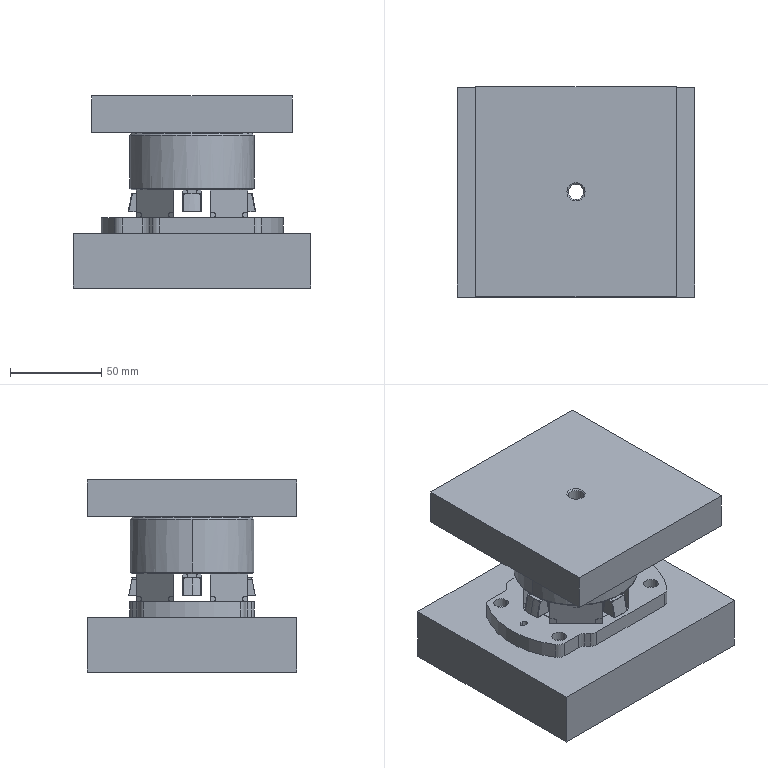NC program | NX | posted with a generic post | part box 130 x 115 x 105.2 mm
Whole program:
N10 G17 G21 G94 G90
(125 , TOOL : ER25-D2.5-23)
N12 T14 M6
N14 G54
N16 G17 G0 G90 X-40.729 Y0. B0. C0. S6500 M3
N18 G43 Z67. H14
N20 G94 G1 Z0.5 F4500.
N22 X-41.25 Z0.473 F1500.
N24 X-39.75 Z0.394
N26 X-41.25 Z0.315
N28 X-39.75 Z0.237
N30 X-41.25 Z0.158
N32 X-39.75 Z0.08
N34 X-41.25 Z0.001
N36 X-39.75 Z-0.078
N38 X-41.25 Z-0.156
N40 X-39.75 Z-0.235
N42 X-41.25 Z-0.313
N44 X-39.75 Z-0.392
N46 X-41.25 Z-0.471
N48 X-39.75 Z-0.549
N50 X-41.25 Z-0.628
N52 X-39.75 Z-0.706
N54 X-41.25 Z-0.785
N56 X-39.75 Z-0.864
N58 X-41.25 Z-0.942
N60 X-39.75 Z-1.021
N62 X-41.25 Z-1.1
N64 X-39.75 Z-1.178
N66 X-41.25 Z-1.257
N68 X-39.75 Z-1.335
N70 X-41.25 Z-1.414
N72 X-39.75 Z-1.493
N74 X-41.25 Z-1.571
N76 X-39.75 Z-1.65
N78 X-41.25 Z-1.728
N80 X-39.75 Z-1.807
N82 X-41.25 Z-1.886
N84 X-39.75 Z-1.964
N86 X-41.25 Z-2.043
N88 X-39.75 Z-2.121
N90 X-41.25 Z-2.2
N92 X-39.75 Z-2.279
N94 X-41.25 Z-2.357
N96 X-39.75 Z-2.436
N98 X-41.25 Z-2.515
N100 X-39.75 Z-2.593
N102 X-41.25 Z-2.672
N104 X-39.75 Z-2.75
N106 X-41.25 Z-2.829
N108 X-39.75 Z-2.908
N110 X-41.25 Z-2.986
N112 X-39.75 Z-3.065
N114 X-41.25 Z-3.143
N116 X-39.75 Z-3.222
N118 X-41.25 Z-3.301
N120 X-39.75 Z-3.379
N122 X-41.25 Z-3.458
N124 X-39.75 Z-3.536
N126 X-41.25 Z-3.615
N128 X-39.75 Z-3.694
N130 X-41.25 Z-3.772
N132 X-39.75 Z-3.851
N134 X-41.25 Z-3.93
N136 X-39.75 Z-4.008
N138 X-41.25 Z-4.087
N140 X-39.75 Z-4.165
N142 X-41.25 Z-4.244
N144 X-39.75 Z-4.323
N146 X-41.25 Z-4.401
N148 X-39.75 Z-4.48
N150 X-41.25 Z-4.558
N152 X-39.75 Z-4.637
N154 X-41.25 Z-4.716
N156 X-39.75 Z-4.794
N158 X-41.25 Z-4.873
N160 X-39.75 Z-4.952
N162 X-41.25 Z-5.03
N164 X-39.75 Z-5.109
N166 X-41.25 Z-5.187
N168 X-39.75 Z-5.266
N170 X-41.25 Z-5.345
N172 X-39.75 Z-5.423
N174 X-41.25 Z-5.502
N176 X-39.75 Z-5.58
N178 X-41.25 Z-5.659
N180 X-39.75 Z-5.738
N182 X-41.25 Z-5.816
N184 X-39.75 Z-5.895
N186 X-41.25 Z-5.973
N188 X-39.75 Z-6.052
N190 X-41.25 Z-6.131
N192 X-39.75 Z-6.209
N194 X-41.25 Z-6.288
N196 X-39.75 Z-6.367
N198 X-41.25 Z-6.445
N200 X-39.75 Z-6.524
N202 X-41.25 Z-6.602
N204 X-39.75 Z-6.681
N206 X-41.25 Z-6.76
N208 X-39.75 Z-6.838
N210 X-41.25 Z-6.917
N212 X-39.75 Z-6.995
N214 X-41.25 Z-7.074
N216 X-39.75 Z-7.153
N218 X-41.25 Z-7.231
N220 X-39.75 Z-7.31
N222 X-41.25 Z-7.388
N224 X-39.75 Z-7.467
N226 X-41.25 Z-7.546
N228 X-39.75 Z-7.624
N230 X-41.25 Z-7.703
N232 X-39.75 Z-7.782
N234 X-41.25 Z-7.86
N236 X-39.75 Z-7.939
N238 X-41.25 Z-8.017
N240 X-39.75 Z-8.096
N242 X-41.25 Z-8.175
N244 X-39.75 Z-8.253
N246 X-41.25 Z-8.332
N248 X-39.75 Z-8.41
N250 X-41.25 Z-8.489
N252 X-39.75 Z-8.568
N254 X-41.25 Z-8.646
N256 X-39.75 Z-8.725
N258 X-41.25 Z-8.803
N260 X-39.75 Z-8.882
N262 X-41.25 Z-8.961
N264 X-40.5 Z-9.
N266 X-39.75
N268 X-41.25
N270 X-40.5
N272 X-40.
N274 Z-8.5
N276 G0 Z67.
N278 M5
(126 , TOOL : ER25-D2.5-23_G)
N280 T15 M6
N282 G54
N284 G17 G0 G90 X-40.623 Y0. B0. C0. S4934 M3
N286 G43 Z67. H15
N288 G94 G1 Z-3. F4500.
N290 G41 X-40.625 Y-0.12 F100. D15
N292 X-40.62 Y-0.159
N294 X-40.602 Y-0.194
N296 X-40.574 Y-0.222
N298 X-40.539 Y-0.24
N300 X-40.5 Y-0.245
N302 X-39.75
N304 G3 X-39.505 Y0. R0.245
N306 X-39.75 Y0.245 R0.245
N308 G1 X-41.25
N310 G3 X-41.495 Y0. R0.245
N312 X-41.25 Y-0.245 R0.245
N314 G1 X-40.5
N316 X-40.
N318 X-39.961 Y-0.24
N320 X-39.926 Y-0.222
N322 X-39.898 Y-0.194
N324 X-39.88 Y-0.159
N326 X-39.875 Y-0.12
N328 G40
N330 X-39.877 Y0.
N332 X-40.623 Y-0.005
N334 G41 X-40.625 Y-0.125
N336 X-40.62 Y-0.164
N338 X-40.602 Y-0.199
N340 X-40.574 Y-0.227
N342 X-40.539 Y-0.245
N344 X-40.5 Y-0.25
N346 X-39.75
N348 G3 X-39.5 Y0. R0.25
N350 X-39.75 Y0.25 R0.25
N352 G1 X-41.25
N354 G3 X-41.5 Y0. R0.25
N356 X-41.25 Y-0.25 R0.25
N358 G1 X-40.5
N360 X-40.
N362 X-39.961 Y-0.245
N364 X-39.926 Y-0.227
N366 X-39.898 Y-0.199
N368 X-39.88 Y-0.164
N370 X-39.875 Y-0.125
N372 G40
N374 X-39.877 Y-0.005
N376 X-40.623 Y0. Z-6. F6000.
N378 G41 X-40.625 Y-0.12 F100.
N380 X-40.62 Y-0.159
N382 X-40.602 Y-0.194
N384 X-40.574 Y-0.222
N386 X-40.539 Y-0.24
N388 X-40.5 Y-0.245
N390 X-39.75
N392 G3 X-39.505 Y0. R0.245
N394 X-39.75 Y0.245 R0.245
N396 G1 X-41.25
N398 G3 X-41.495 Y0. R0.245
N400 X-41.25 Y-0.245 R0.245
N402 G1 X-40.5
N404 X-40.
N406 X-39.961 Y-0.24
N408 X-39.926 Y-0.222
N410 X-39.898 Y-0.194
N412 X-39.88 Y-0.159
N414 X-39.875 Y-0.12
N416 G40
N418 X-39.877 Y0.
N420 X-40.623 Y-0.005
N422 G41 X-40.625 Y-0.125
N424 X-40.62 Y-0.164
N426 X-40.602 Y-0.199
N428 X-40.574 Y-0.227
N430 X-40.539 Y-0.245
N432 X-40.5 Y-0.25
N434 X-39.75
N436 G3 X-39.5 Y0. R0.25
N438 X-39.75 Y0.25 R0.25
N440 G1 X-41.25
N442 G3 X-41.5 Y0. R0.25
N444 X-41.25 Y-0.25 R0.25
N446 G1 X-40.5
N448 X-40.
N450 X-39.961 Y-0.245
N452 X-39.926 Y-0.227
N454 X-39.898 Y-0.199
N456 X-39.88 Y-0.164
N458 X-39.875 Y-0.125
N460 G40
N462 X-39.877 Y-0.005
N464 X-40.623 Y0. Z-9. F6000.
N466 G41 X-40.625 Y-0.12 F100.
N468 X-40.62 Y-0.159
N470 X-40.602 Y-0.194
N472 X-40.574 Y-0.222
N474 X-40.539 Y-0.24
N476 X-40.5 Y-0.245
N478 X-39.75
N480 G3 X-39.505 Y0. R0.245
N482 X-39.75 Y0.245 R0.245
N484 G1 X-41.25
N486 G3 X-41.495 Y0. R0.245
N488 X-41.25 Y-0.245 R0.245
N490 G1 X-40.5
N492 X-40.
N494 X-39.961 Y-0.24
N496 X-39.926 Y-0.222
N498 X-39.898 Y-0.194
N500 X-39.88 Y-0.159
N502 X-39.875 Y-0.12
N504 G40
N506 X-39.877 Y0.
N508 X-40.623 Y-0.005
N510 G41 X-40.625 Y-0.125
N512 X-40.62 Y-0.164
N514 X-40.602 Y-0.199
N516 X-40.574 Y-0.227
N518 X-40.539 Y-0.245
N520 X-40.5 Y-0.25
N522 X-39.75
N524 G3 X-39.5 Y0. R0.25
N526 X-39.75 Y0.25 R0.25
N528 G1 X-41.25
N530 G3 X-41.5 Y0. R0.25
N532 X-41.25 Y-0.25 R0.25
N534 G1 X-40.5
N536 X-40.
N538 X-39.961 Y-0.245
N540 X-39.926 Y-0.227
N542 X-39.898 Y-0.199
N544 X-39.88 Y-0.164
N546 X-39.875 Y-0.125
N548 G40
N550 X-39.877 Y-0.005
N552 G0 Z67.
N554 M5
(ADAPTIVE_MILLING , TOOL : ER25-D10-50)
N556 T04 M6
N558 G54
N560 G17 G0 G90 X61.557 Y1.041 B0. C0. S6500 M3
N562 G43 Z67. H4
N564 Z-6.
N566 G94 G1 X61.407 Y1.026 Z-6.937 F2000.
N568 X61.258 Y1.01 Z-7.308
N570 X61.109 Y0.994 Z-7.58
N572 X60.96 Y0.978 Z-7.8
N574 X60.811 Y0.963 Z-7.984
N576 X60.662 Y0.947 Z-8.142
N578 X60.512 Y0.931 Z-8.28
N580 X60.363 Y0.915 Z-8.4
N582 X60.214 Y0.899 Z-8.505
N584 X60.065 Y0.884 Z-8.598
N586 X59.916 Y0.868 Z-8.679
N588 X59.767 Y0.852 Z-8.75
N590 X59.617 Y0.836 Z-8.81
N592 X59.468 Y0.821 Z-8.862
N594 X59.319 Y0.805 Z-8.905
N596 X59.17 Y0.789 Z-8.939
N598 X59.021 Y0.773 Z-8.966
N600 X58.872 Y0.758 Z-8.985
N602 X58.722 Y0.742 Z-8.996
N604 X58.573 Y0.726 Z-9.
N606 X56.835 Y0.542
N608 G3 X56.075 Y0.057 R1.012
N610 X55.469 Y-1.557 R5.121
N612 X55.189 Y-3.496 R6.542
N614 G1 X54.855 Y-7.003
N616 X54.298 Y-10.48
N618 X53.52 Y-13.916
N620 X52.526 Y-17.295
N622 X51.318 Y-20.604
N624 X49.903 Y-23.829
N626 X48.285 Y-26.957
N628 X46.47 Y-29.976
N630 X44.468 Y-32.874
N632 X42.285 Y-35.638
N634 G2 X39.627 Y-38.203 R45.056
N636 X30.654 Y-45.533 R68.05
N638 X-44.698 Y-31.875 R54.912
N640 X-45.9 Y-30.686 R23.81
N642 G1 X-46.779 Y-29.493
N644 X-48.53 Y-26.513
N646 X-50.091 Y-23.43
N648 X-51.457 Y-20.256
N650 X-52.621 Y-17.002
N652 X-53.581 Y-13.682
N654 X-54.331 Y-10.308
N656 X-54.869 Y-6.894
N658 X-55.192 Y-3.454
N660 X-55.3 Y0.
N662 X-55.192 Y3.455
N664 X-54.868 Y6.895
N666 X-54.331 Y10.309
N668 X-53.581 Y13.683
N670 X-52.621 Y17.003
N672 X-51.456 Y20.257
N674 X-50.091 Y23.431
N676 X-48.529 Y26.514
N678 X-46.778 Y29.494
N680 G2 X-44.339 Y32.598 R57.555
N682 X-36.468 Y41.03 R68.244
N684 X39.85 Y37.753 R54.906
N686 G1 X41.244 Y36.706
N688 X42.286 Y35.637
N690 X44.466 Y32.877
N692 X46.466 Y29.983
N694 X48.278 Y26.968
N696 X49.895 Y23.844
N698 X51.31 Y20.624
N700 X52.518 Y17.319
N702 X53.513 Y13.945
N704 X54.291 Y10.515
N706 X54.85 Y7.042
N708 X55.187 Y3.54
N710 X55.3 Y0.025
N712 X55.21 Y-2.849
N714 G3 X55.811 Y-3.803 R1.029
N716 G1 X57.534 Y-4.748 Z-8.9
N718 X57.745 Y-4.864 F15000.
N720 X57.951 Y-4.988
N722 G2 X58.335 Y-5.975 R1.001
N724 G1 X57.958 Y-7.984
N726 X57.57 Y-9.991
N728 G2 X56.311 Y-14.938 R57.161
N730 X54.364 Y-20.753 R77.546
N732 X50.136 Y-29.595 R62.207
N734 X48.222 Y-32.737 R76.126
N736 G1 X45.662 Y-36.707
N738 G2 X44.586 Y-37.137 R1.
N740 G1 X44.302 Y-37.068
N742 X42.392 Y-36.605 Z-9. F2000.
N744 X42.167 Y-36.55
N746 X41.939 Y-36.506
N748 G3 X41.242 Y-36.707 R1.004
N750 G1 X40.056 Y-37.614
N752 G3 X36.023 Y-40.298 R25.388
N754 G2 X28.458 Y-45.679 R86.812
N756 X-42.013 Y-33.615 R53.839
N758 G3 X-42.38 Y-33.353 R1.719
N760 G1 X-43.678 Y-32.637
N762 X-44.774 Y-31.806
N764 G3 X-46.314 Y-32.252 R1.
N766 X-46.255 Y-33.092 Z-8.956 R1.045
N768 G1 X-45.811 Y-34.095 Z-8.9
N770 X-45.012 Y-35.895 F15000.
N772 G3 X-44.774 Y-36.227 R1.06
N774 G1 X-42.966 Y-37.885
N776 X-41.136 Y-39.519
N778 X-40.204 Y-40.315
N780 X-39.263 Y-41.103
N782 X-37.604 Y-42.468
N784 X-35.937 Y-43.824
N786 G3 X-29.941 Y-48.068 R67.977
N788 X-26.259 Y-50.265 R58.863
N790 X-20.692 Y-52.821 R51.545
N792 X-11.888 Y-55.431 R52.347
N794 X-4.629 Y-56.645 R87.095
N796 X2.098 Y-56.811 R36.217
N798 X9.998 Y-55.815 R57.149
N800 X16.942 Y-54.12 R66.102
N802 X22.299 Y-52.122 R49.474
N804 X28.844 Y-48.784 R54.765
N806 G1 X32.007 Y-46.896
N808 X35.161 Y-44.995
N810 X38.854 Y-42.703
N812 G3 X39.261 Y-42.207 R1.007
N814 G1 X39.894 Y-40.526
N816 X40.297 Y-39.439 Z-8.959 F2000.
N818 G3 X40.209 Y-38.661 Z-9. R1.
N820 X38.854 Y-38.283 R1.
N822 G1 X36.961 Y-39.041
N824 G3 X33.434 Y-41.169 R28.709
N826 G2 X25.898 Y-45.947 R97.732
N828 X-39.701 Y-34.694 R52.812
N830 G3 X-40.475 Y-34.011 R2.805
N832 G2 X-42.38 Y-33.353 R14.859
N834 G3 X-43.729 Y-34.201 R1.
N836 X-43.441 Y-35. Z-8.955 R1.044
N838 G1 X-42.742 Y-35.835 Z-8.9
N840 X-41.994 Y-36.733 F15000.
N842 X-41.236 Y-37.623
N844 X-39.689 Y-39.111
N846 X-38.134 Y-40.592
N848 G3 X-33.759 Y-44.37 R73.242
N850 X-29.403 Y-47.292 R36.344
N852 X-25.96 Y-49.209 R99.842
N854 X-20.624 Y-51.634 R55.888
N856 X-10.848 Y-54.548 R53.534
N858 G1 X-9.843 Y-54.729
N860 X-8.835 Y-54.893
N862 X-6.044 Y-55.302
N864 G3 X2.746 Y-55.629 R48.097
N866 G1 X5.461 Y-55.47
N868 G3 X10.647 Y-54.702 R37.882
N870 X19.016 Y-52.314 R72.877
N872 X26.164 Y-49.099 R47.371
N874 X33.331 Y-44.924 R163.072
N876 G1 X36.211 Y-43.139
N878 X36.353 Y-43.031
N880 X36.476 Y-42.901
N882 X37.696 Y-41.321
N884 X38.403 Y-40.397 Z-8.959 F2000.
N886 G3 X38.548 Y-39.632 Z-9. R1.
N888 X37.355 Y-38.87 R1.
N890 X33.268 Y-40.392 R11.961
N892 X27.346 Y-43.927 R432.569
N894 G2 X10.647 Y-50.521 R55.409
N896 X-37.562 Y-35.435 R51.68
N898 G3 X-38.808 Y-34.337 R8.034
N900 X-39.545 Y-34.193 R1.678
N902 G1 X-40.644 Y-33.952
N904 G3 X-41.833 Y-34.702 R1.
N906 X-41.583 Y-35.625 Z-8.949 R1.043
N908 G1 X-40.981 Y-36.386 Z-8.9
N910 X-40.286 Y-37.271 F15000.
N912 X-39.58 Y-38.148
N914 X-39.5 Y-38.222
N916 X-36.886 Y-40.358
N918 X-34.261 Y-42.481
N920 G3 X-29.456 Y-45.941 R68.449
N922 X-21.321 Y-50.19 R50.428
N924 X-16.339 Y-52.028 R78.714
N926 X-6.364 Y-54.143 R51.577
N928 X-0.164 Y-54.665 R89.323
N930 X4.023 Y-54.462 R25.809
N932 G1 X6.335 Y-54.161
N934 X8.645 Y-53.848
N936 G3 X17.791 Y-51.57 R48.335
N938 X23.442 Y-49.21 R49.142
N940 G1 X27.022 Y-47.448
N942 X30.594 Y-45.67
N944 X32.794 Y-44.544
N946 X34.991 Y-43.409
N948 G3 X35.329 Y-43.124 R1.042
N950 G1 X36.493 Y-41.585
N952 X37.188 Y-40.658 Z-8.959 F2000.
N954 G3 X37.324 Y-39.887 Z-9. R1.
N956 X36.135 Y-39.139 R1.
N958 G2 X35.149 Y-39.246 R5.011
N960 G3 X32.094 Y-40.252 R10.348
N962 X26.499 Y-43.263 R113.682
N964 G2 X13.481 Y-48.714 R59.152
N966 X-35.356 Y-36.124 R50.6
N968 G3 X-37.398 Y-34.418 R13.365
N970 X-38.066 Y-34.3 R1.369
N972 G1 X-39.188 Y-34.219
N974 G3 X-40.221 Y-34.938 R1.
N976 X-40.011 Y-35.884 Z-8.949 R1.041
N978 G1 X-39.446 Y-36.655 Z-8.9
N980 X-38.827 Y-37.506 F15000.
N982 X-38.198 Y-38.351
N984 X-38.044 Y-38.489
N986 X-34.819 Y-40.837
N988 X-31.584 Y-43.171
N990 G3 X-26.11 Y-46.671 R77.601
N992 X-20.821 Y-49.235 R44.189
N994 X-16.907 Y-50.673 R67.048
N996 X-8.393 Y-52.981 R67.15
N998 X-0.743 Y-53.574 R33.294
N1000 X6.597 Y-53.048 R84.732
N1002 X13.209 Y-51.772 R48.024
N1004 X20.174 Y-49.444 R51.333
N1006 X34.005 Y-43.516 R529.24
N1008 X34.426 Y-43.167 R1.013
N1010 G1 X35.434 Y-41.701
N1012 X36.083 Y-40.746 Z-8.959 F2000.
N1014 G3 X36.182 Y-39.966 Z-9. R1.
N1016 X35.149 Y-39.246 R1.
N1018 X33.391 Y-39.349 R86.82
N1020 X29.731 Y-40.591 R14.09
N1022 X23.318 Y-43.785 R423.321
N1024 G2 X7.788 Y-48.833 R54.739
N1026 X-33.005 Y-36.822 R49.472
N1028 G3 X-35.615 Y-34.658 R29.808
N1030 X-36.414 Y-34.3 R1.797
N1032 G1 X-37.914
N1034 G3 X-38.873 Y-35.016 R1.
N1036 X-38.678 Y-35.953 Z-8.949 R1.043
N1038 G1 X-38.122 Y-36.747 Z-8.9
N1040 X-37.021 Y-38.321 F15000.
N1042 X-36.905 Y-38.455
N1044 X-36.77 Y-38.57
N1046 X-34.249 Y-40.316
N1048 X-31.719 Y-42.049
N1050 G3 X-21.548 Y-47.706 R74.879
N1052 X-8.686 Y-51.617 R50.172
N1054 X-1.065 Y-52.413 R69.958
N1056 X5.955 Y-52.076 R39.103
N1058 X16.892 Y-49.58 R55.986
N1060 X23.525 Y-46.91 R70.317
N1062 G1 X31.699 Y-43.128
N1064 X31.868 Y-43.028
N1066 X33.6 Y-41.763
N1068 X34.553 Y-41.062 Z-8.96 F2000.
N1070 G3 X34.905 Y-40.387 Z-9. R1.
N1072 X33.909 Y-39.3 R1.
N1074 X31.774 Y-39.35 R16.816
N1076 X27.681 Y-40.676 R16.703
N1078 G1 X21.146 Y-43.668
N1080 G2 X5.545 Y-48.036 R53.459
N1082 X-31.279 Y-36.884 R48.475
N1084 G3 X-34.142 Y-34.647 R35.773
N1086 X-34.94 Y-34.3 R1.842
N1088 G1 X-36.44
N1090 G3 X-37.398 Y-35.013 R1.
N1092 X-37.208 Y-35.948 Z-8.95 R1.043
N1094 G1 X-36.656 Y-36.749 Z-8.9
N1096 X-35.597 Y-38.285 F15000.
N1098 G3 X-35.296 Y-38.57 R1.056
N1100 G1 X-27.445 Y-43.378
N1102 G3 X-17.335 Y-48.238 R54.627
N1104 X-10.45 Y-50.149 R49.024
N1106 G1 X-7.743 Y-50.694
N1108 X-5.033 Y-51.227
N1110 X-4.23 Y-51.378
N1112 X-3.424 Y-51.515
N1114 G3 X-1.393 Y-51.58 R9.81
N1116 G1 X0.749 Y-51.424
N1118 X2.89 Y-51.259
N1120 G3 X8.768 Y-50.518 R77.791
N1122 X19.552 Y-47.434 R51.222
N1124 G1 X30.074 Y-43.128
N1126 X30.183 Y-43.073
N1128 X30.287 Y-43.009
N1130 X31.981 Y-41.764
N1132 X32.93 Y-41.06 Z-8.96 F2000.
N1134 G3 X33.28 Y-40.383 Z-9. R1.
N1136 X32.284 Y-39.3 R1.
N1138 X30.037 Y-39.344 R20.664
N1140 X26.038 Y-40.515 R17.729
N1142 G1 X19.466 Y-43.268
N1144 G2 X4.363 Y-47.058 R53.087
N1146 X-29.273 Y-37.107 R47.391
N1148 G3 X-32.49 Y-34.701 R57.335
N1150 X-33.385 Y-34.3 R2.147
N1152 G1 X-35.01
N1154 G3 X-36.008 Y-35.373 R1.
N1156 X-35.521 Y-36.164 Z-8.951 R1.04
N1158 G1 X-34.71 Y-36.75 Z-8.9
N1160 X-32.8 Y-38.128 F15000.
N1162 X-31.262 Y-39.363
N1164 X-29.712 Y-40.585
N1166 G3 X-24.775 Y-43.729 R36.797
N1168 X-14.859 Y-47.939 R54.835
N1170 X-10.461 Y-49.046 R44.725
N1172 X-0.859 Y-50.146 R54.155
N1174 X11.784 Y-48.792 R52.599
N1176 X15.551 Y-47.71 R41.52
N1178 X23.273 Y-45.018 R309.641
N1180 G1 X25.8 Y-44.078
N1182 X28.324 Y-43.128
N1184 X28.448 Y-43.069
N1186 X28.566 Y-42.997
N1188 X30.234 Y-41.765
N1190 X31.182 Y-41.058 Z-8.96 F2000.
N1192 G3 X31.53 Y-40.382 Z-9. R1.
N1194 X30.534 Y-39.3 R1.
N1196 X28.293 Y-39.318 R109.815
N1198 X24.263 Y-40.359 R17.754
N1200 G1 X17.722 Y-42.844
N1202 G2 X3.121 Y-46.056 R52.472
N1204 X-27.488 Y-37.091 R46.395
N1206 G3 X-30.899 Y-34.671 R77.132
N1208 X-31.743 Y-34.3 R2.12
N1210 G1 X-33.493
N1212 G3 X-34.491 Y-35.372 R1.
N1214 X-34.005 Y-36.164 Z-8.951 R1.04
N1216 G1 X-33.194 Y-36.75 Z-8.9
N1218 X-31.283 Y-38.128 F15000.
N1220 X-28.63 Y-39.918
N1222 X-25.968 Y-41.694
N1224 G3 X-20.44 Y-44.64 R39.556
N1226 X-11.762 Y-47.631 R53.177
N1228 X-6.267 Y-48.693 R56.402
N1230 X0.575 Y-49.047 R39.156
N1232 G1 X2.003 Y-48.991
N1234 X3.431 Y-48.925
N1236 G3 X14.456 Y-46.918 R47.061
N1238 G1 X18.136 Y-45.783
N1240 X21.808 Y-44.621
N1242 X26.324 Y-43.128
N1244 X26.469 Y-43.064
N1246 X26.605 Y-42.981
N1248 X28.241 Y-41.765
N1250 X29.185 Y-41.056 Z-8.96 F2000.
N1252 G3 X29.531 Y-40.376 Z-9. R1.
N1254 X28.534 Y-39.3 R1.
N1256 X26.154 Y-39.318 R115.941
N1258 X21.947 Y-40.33 R19.912
N1260 G2 X14.623 Y-42.791 R276.472
N1262 X-2.52 Y-44.986 R48.992
N1264 X-25.984 Y-36.827 R45.591
N1266 G3 X-29.368 Y-34.563 R68.185
N1268 X-30.047 Y-34.3 R1.79
N1270 G1 X-31.797
N1272 G3 X-32.795 Y-35.372 R1.
N1274 X-32.309 Y-36.164 Z-8.951 R1.04
N1276 G1 X-31.498 Y-36.75 Z-8.9
N1278 X-29.587 Y-38.128 F15000.
N1280 X-27.625 Y-39.388
N1282 X-25.656 Y-40.635
N1284 G3 X-15.003 Y-45.574 R50.533
N1286 G1 X-14.067 Y-45.866
N1288 X-13.126 Y-46.141
N1290 X-11.516 Y-46.593
N1292 X-9.901 Y-47.029
N1294 G3 X-1.12 Y-48.02 R33.308
N1296 G1 X0.598 Y-47.985
N1298 X2.316 Y-47.939
N1300 G3 X8.646 Y-47.236 R44.998
N1302 G1 X9.847 Y-46.989
N1304 X11.039 Y-46.708
N1306 G3 X20.594 Y-44.164 R282.274
N1308 G1 X24.199 Y-43.128
N1310 X24.367 Y-43.061
N1312 X24.523 Y-42.967
N1314 X26.124 Y-41.764
N1316 X27.063 Y-41.053 Z-8.96 F2000.
N1318 G3 X27.406 Y-40.369 Z-9. R1.
N1320 X26.409 Y-39.3 R1.
N1322 X23.61 Y-39.338 R35.028
N1324 X19.003 Y-40.406 R26.148
N1326 G2 X10.9 Y-42.696 R117.782
N1328 X-11.009 Y-42.548 R45.806
N1330 X-20.242 Y-39.019 R47.246
N1332 X-24.425 Y-36.98 R10.054
N1334 G3 X-28.007 Y-34.42 R26.513
N1336 X-28.42 Y-34.3 R3.816
N1338 G1 X-30.17
N1340 G3 X-31.266 Y-35.49 R1.1
N1342 X-30.57 Y-36.429 Z-8.937 R1.127
N1344 G1 X-29.91 Y-36.751 Z-8.9
N1346 X-26.519 Y-38.407 F15000.
N1348 X-25.438 Y-38.93 Z-8.961 F2000.
N1350 G3 X-24.692 Y-38.966 Z-9. R1.102
N1352 X-24.294 Y-37.088 R1.1
N1354 G2 X-26.715 Y-34.78 R33.235
N1356 G3 X-27.635 Y-34.3 R1.46
N1358 G1 X-28.51
N1360 G3 X-28.679 Y-36.487 R1.1
N1362 G1 X-27.662 Y-36.645
N1364 G3 X-26.715 Y-34.78 R1.1
N1366 X-27.553 Y-34.308 R1.222
N1368 X-28.535 Y-34.837 R1.001
N1370 X-28.603 Y-35.623 Z-8.959 R1.06
N1372 G1 X-28.342 Y-36.748 Z-8.9
N1374 X-28.032 Y-38.085 F15000.
N1376 G3 X-27.553 Y-38.729 R1.003
N1378 G1 X-26.132 Y-39.538
N1380 X-24.705 Y-40.338
N1382 G3 X-21.005 Y-42.058 R35.003
N1384 G1 X-18.805 Y-42.932
N1386 X-16.599 Y-43.789
N1388 G3 X-9.975 Y-45.736 R51.379
N1390 X-3.951 Y-46.896 R81.762
N1392 X2.131 Y-46.99 R22.278
N1394 X6.735 Y-46.384 R138.174
N1396 X13.615 Y-45.061 R92.691
N1398 G1 X21.949 Y-43.128
N1400 G3 X22.328 Y-42.95 R1.053
N1402 G1 X23.886 Y-41.764
N1404 X24.818 Y-41.048 Z-8.96 F2000.
N1406 G3 X25.157 Y-40.36 Z-9. R1.
N1408 X24.159 Y-39.3 R1.
N1410 X21.131 Y-39.318 R142.895
N1412 X16.511 Y-40.232 R29.053
N1414 G2 X8.207 Y-42.154 R98.209
N1416 X-13.988 Y-40.488 R44.289
N1418 X-17.022 Y-39.326 R128.817
N1420 G3 X-17.929 Y-39.3 R5.146
N1422 G2 X-20.255 Y-39.017 R10.98
N1424 G3 X-21.405 Y-40.296 R1.
N1426 X-20.953 Y-40.867 Z-8.962 R1.064
N1428 G1 X-19.958 Y-41.574 Z-8.9
N1430 X-18.393 Y-42.687 F15000.
N1432 X-18.226 Y-42.781
N1434 X-18.045 Y-42.845
N1436 X-14.861 Y-43.605
N1438 X-11.675 Y-44.353
N1440 G3 X-3.113 Y-45.641 R66.52
N1442 X1.293 Y-45.777 R40.191
N1444 X3.736 Y-45.608 R34.265
N1446 X12.235 Y-44.416 R104.522
N1448 G1 X19.199 Y-43.128
N1450 G3 X19.627 Y-42.937 R1.025
N1452 G1 X21.146 Y-41.766
N1454 X22.073 Y-41.044 Z-8.96 F2000.
N1456 G3 X22.407 Y-40.353 Z-9. R1.
N1458 X21.409 Y-39.3 R1.
N1460 X17.997 Y-39.322 R79.243
N1462 X13.367 Y-40.094 R38.307
N1464 G2 X3.989 Y-41.606 R72.689
N1466 X-13.988 Y-39.32 R43.037
N1468 G1 X-14.114 Y-39.3
N1470 X-17.239
N1472 G3 X-17.572 Y-41.243 R1.
N1474 G1 X-15.674 Y-41.753 Z-8.9
N1476 X-15.151 Y-41.895 F15000.
N1478 X-14.624 Y-42.025
N1480 X-14.504 Y-42.035
N1482 X16.475 Y-42.65
N1484 G3 X17.071 Y-42.467 R1.008
N1486 G1 X18.067 Y-41.765
N1488 X19.039 Y-41.073 Z-8.961 F2000.
N1490 G3 X19.402 Y-40.415 Z-9. R1.
N1492 X18.409 Y-39.3 R1.
N1494 X14.105 Y-39.322 R100.131
N1496 X8.308 Y-40.067 R92.546
N1498 G2 X-3.532 Y-40.482 R50.963
N1500 X-10.297 Y-39.3 R44.352
N1502 G1 X-14.172
N1504 G3 X-14.501 Y-41.244 R1.
N1506 G1 X-12.604 Y-41.753 Z-8.9
N1508 X-12.081 Y-41.896 F15000.
N1510 X-11.554 Y-42.025
N1512 X-11.437 Y-42.035
N1514 X12.6 Y-42.65
N1516 G3 X13.203 Y-42.466 R1.008
N1518 G1 X14.195 Y-41.765
N1520 X15.166 Y-41.072 Z-8.961 F2000.
N1522 G3 X15.527 Y-40.413 Z-9. R1.
N1524 X14.534 Y-39.3 R1.
N1526 X7.801 Y-39.328 R211.445
N1528 G2 X0.23 Y-39.591 R110.463
N1530 X-4.238 Y-39.3 R48.732
N1532 G1 X-10.363
N1534 G3 X-10.707 Y-41.239 R1.
N1536 G1 X-8.811 Y-41.753 Z-8.9
N1538 X-8.287 Y-41.897 F15000.
N1540 X-7.759 Y-42.026
N1542 X-7.628 Y-42.035
N1544 X5.799
N1546 X5.929 Y-42.024
N1548 X6.058 Y-42.001
N1550 X6.956 Y-41.759
N1552 X8.853 Y-41.248 Z-9. F2000.
N1554 G3 X8.534 Y-39.3 R1.
N1556 G1 X-4.341
N1558 G3 X-5.178 Y-39.753 R1.001
N1560 G1 X-5.41 Y-40.108
N1562 X-6.486 Y-41.752 Z-8.9
N1564 X-6.716 Y-42.086 F15000.
N1566 G2 X-7.467 Y-42.426 R1.002
N1568 G1 X-10.73 Y-42.429
N1570 X-13.992 Y-42.415
N1572 G2 X-23.89 Y-41.13 R46.488
N1574 G1 X-40.603 Y-37.099
N1576 G2 X-44.004 Y-35.788 R13.96
N1578 X-46.193 Y-34.446 R17.549
N1580 X-48.277 Y-32.402 R9.475
N1582 X-49.803 Y-30.269 R47.735
N1584 X-51.519 Y-27.228 R26.134
N1586 G1 X-52.358 Y-25.475
N1588 X-53.167 Y-23.709
N1590 G2 X-56.58 Y-13.45 R57.575
N1592 X-57.827 Y-6.21 R57.255
N1594 X-58.244 Y-1.934 R120.419
N1596 X-58.361 Y0.515 R35.9
N1598 X-58.221 Y2.959 R21.656
N1600 G1 X-57.885 Y5.906
N1602 X-57.532 Y8.85
N1604 G2 X-55.099 Y18.749 R50.063
N1606 G1 X-54.45 Y20.498
N1608 X-53.78 Y22.24
N1610 G2 X-52.042 Y26.07 R48.964
N1612 G1 X-50.946 Y28.22
N1614 X-50.566 Y28.887
N1616 X-50.169 Y29.544
N1618 G2 X-49.329 Y30.031 R1.055
N1620 G1 X-47.381 Y30.283 Z-9. F2000.
N1622 X-46.866 Y30.346
N1624 X-46.353 Y30.424
N1626 G3 X-45.899 Y30.688 R1.016
N1628 G1 X-44.858 Y31.743
N1630 G3 X-41.33 Y34.852 R25.349
N1632 G2 X-34.59 Y41.234 R89.377
N1634 X37.063 Y39.016 R53.858
N1636 G1 X37.357 Y38.869
N1638 X38.753 Y38.339
N1640 X39.955 Y37.67
N1642 G3 X41.415 Y38.769 R1.
N1644 X41.14 Y39.266 Z-8.971 R1.099
N1646 G1 X40.235 Y40.321 Z-8.9
N1648 X38.98 Y41.784 F15000.
N1650 X38.81 Y41.94
N1652 X36.086 Y43.933
N1654 X33.352 Y45.912
N1656 G3 X26.136 Y50.317 R68.704
N1658 X14.619 Y54.799 R56.238
N1660 X8.677 Y56.334 R193.946
N1662 X2.624 Y56.997 R24.022
N1664 X-3.5 Y56.704 R75.484
N1666 X-7.151 Y56.261 R68.391
N1668 G1 X-9.071 Y55.976
N1670 X-10.989 Y55.677
N1672 G3 X-14.965 Y54.755 R36.259
N1674 X-22.091 Y52.236 R71.08
N1676 X-27.941 Y49.333 R55.367
N1678 X-34.423 Y45.069 R58.715
N1680 X-37.201 Y42.818 R71.051
N1682 X-40.665 Y39.793 R143.386
N1684 G1 X-43.762 Y36.993
N1686 G3 X-44.006 Y36.656 R1.055
N1688 G1 X-44.815 Y34.826
N1690 X-45.303 Y33.711 Z-8.962 F2000.
N1692 G3 X-45.287 Y32.982 Z-9. R1.001
N1694 X-43.762 Y32.573 R1.
N1696 G1 X-41.921 Y33.635
N1698 G3 X-38.846 Y36.123 R29.356
N1700 G2 X-32.138 Y41.824 R100.772
N1702 X34.599 Y39.789 R52.829
N1704 G3 X35.455 Y39.24 R2.474
N1706 G2 X37.357 Y38.869 R13.902
N1708 G3 X38.544 Y39.604 R1.
N1710 X38.306 Y40.533 Z-8.949 R1.042
N1712 G1 X37.715 Y41.299 Z-8.9
N1714 X36.483 Y42.897 F15000.
N1716 X36.358 Y43.029
N1718 X36.213 Y43.139
N1720 X28.884 Y47.625
N1722 G3 X20.068 Y51.885 R48.59
N1724 X14.242 Y53.793 R75.344
N1726 X9.808 Y54.887 R91.965
N1728 X0.989 Y55.735 R38.523
N1730 G1 X-0.984 Y55.699
N1732 X-2.958 Y55.649
N1734 G3 X-8.175 Y55.101 R41.18
N1736 X-17.106 Y52.938 R65.449
N1738 X-24.663 Y49.853 R52.003
N1740 X-31.495 Y45.82 R60.957
N1742 X-39.364 Y40.069 R250.711
N1744 G1 X-42.378 Y37.774
N1746 G3 X-42.714 Y37.314 R1.011
N1748 G1 X-43.314 Y35.633
N1750 X-43.692 Y34.553 Z-8.958 F2000.
N1752 G3 X-43.582 Y33.764 Z-9. R1.
N1754 X-42.378 Y33.354 R1.
N1756 X-38.548 Y35.407 R12.068
N1758 X-33.301 Y39.614 R314.253
N1760 G2 X-17.648 Y48.522 R55.67
N1762 X32.422 Y40.199 R51.721
N1764 G3 X33.737 Y39.348 R5.889
N1766 X34.41 Y39.3 R2.309
N1768 G1 X35.657 Y39.209
N1770 G3 X36.686 Y39.916 R1.
N1772 X36.489 Y40.864 Z-8.949 R1.041
N1774 G1 X35.935 Y41.644 Z-8.9
N1776 X34.841 Y43.184 F15000.
N1778 G3 X34.512 Y43.479 R1.042
N1780 G1 X31.833 Y44.975
N1782 X29.147 Y46.458
N1784 G3 X22.527 Y49.67 R92.874
N1786 X17.051 Y51.826 R62.328
N1788 X12.68 Y53.029 R44.031
N1790 X6.644 Y54.073 R54.038
N1792 G1 X4.664 Y54.304
N1794 X2.682 Y54.517
N1796 G3 X-4.35 Y54.504 R39.384
N1798 X-11.602 Y53.337 R47.26
N1800 X-23.003 Y49.471 R64.656
N1802 X-28.048 Y46.786 R47.361
N1804 X-34.115 Y42.636 R61.248
N1806 G1 X-39.947 Y38.108
N1808 X-40.104 Y37.956
N1810 X-41.484 Y36.291
N1812 X-42.253 Y35.357 Z-8.962 F2000.
N1814 G3 X-42.435 Y34.644 Z-9. R1.001
N1816 X-41.091 Y33.838 R1.
N1818 X-39.675 Y34.212 R19.972
N1820 X-36.387 Y36.097 R15.5
N1822 G1 X-30.552 Y40.408
N1824 G2 X-14.007 Y48.561 R53.979
N1826 X30.314 Y40.462 R50.729
N1828 G3 X32.06 Y39.363 R12.498
N1830 G1 X32.338 Y39.3
N1832 X34.088
N1834 G3 X35.085 Y40.372 R1.
N1836 X34.599 Y41.164 Z-8.951 R1.04
N1838 G1 X33.788 Y41.75 Z-8.9
N1840 X31.877 Y43.128 F15000.
N1842 X30.157 Y44.232
N1844 X28.429 Y45.325
N1846 G3 X23.947 Y47.769 R50.972
N1848 X20.04 Y49.542 R62.124
N1850 X11.254 Y52.202 R52.684
N1852 G1 X7.651 Y52.951
N1854 G3 X4.627 Y53.466 R58.126
N1856 X1.574 Y53.607 R19.058
N1858 G1 X-1.319 Y53.51
N1860 X-4.21 Y53.395
N1862 G3 X-10.006 Y52.572 R37.284
N1864 X-15.556 Y51.18 R72.868
N1866 X-19.395 Y49.791 R38.301
N1868 X-22.955 Y48.239 R98.411
N1870 X-27.641 Y45.746 R55.579
N1872 X-31.796 Y43.14 R86.865
N1874 G1 X-38.992 Y38.333
N1876 X-39.117 Y38.232
N1878 X-39.226 Y38.115
N1880 X-40.471 Y36.514
N1882 X-41.18 Y35.593 Z-8.959 F2000.
N1884 G3 X-41.328 Y34.828 Z-9. R1.
N1886 X-40.136 Y34.063 R1.
N1888 G2 X-38.782 Y34.299 R18.736
N1890 G3 X-35.528 Y35.802 R11.895
N1892 X-30.027 Y39.548 R143.182
N1894 G2 X-17.552 Y46.234 R57.929
N1896 X27.658 Y40.998 R49.505
N1898 G3 X30.261 Y39.381 R27.437
N1900 G1 X30.594 Y39.3
N1902 X32.344
N1904 G3 X33.342 Y40.369 R1.
N1906 X32.857 Y41.163 Z-8.951 R1.04
N1908 G1 X32.048 Y41.75 Z-8.9
N1910 X30.235 Y43.064 F15000.
N1912 X30.134 Y43.128
N1914 X27.275 Y44.721
N1916 X24.408 Y46.299
N1918 G3 X16.461 Y49.721 R55.769
N1920 X9.813 Y51.382 R42.391
N1922 X3.739 Y52.195 R74.734
N1924 X-0.545 Y52.417 R54.164
N1926 X-8.123 Y51.795 R44.168
N1928 X-13.838 Y50.493 R50.922
N1930 X-25.169 Y45.893 R53.669
N1932 X-33.722 Y41.075 R297.682
N1934 G1 X-38.15 Y38.481
N1936 G3 X-38.458 Y38.2 R1.054
N1938 G1 X-39.554 Y36.666
N1940 X-40.218 Y35.727 Z-8.959 F2000.
N1942 G3 X-40.33 Y34.944 Z-9. R1.
N1944 X-39.294 Y34.211 R1.
N1946 X-37.259 Y34.443 R11.471
N1948 X-33.624 Y36.1 R14.788
N1950 X-27.461 Y40.029 R350.93
N1952 G2 X-13.733 Y46.367 R54.947
N1954 X25.929 Y40.829 R48.455
N1956 G3 X28.463 Y39.358 R27.686
N1958 G1 X28.726 Y39.3
N1960 X30.601
N1962 G3 X31.599 Y40.367 R1.
N1964 X31.116 Y41.162 Z-8.951 R1.04
N1966 G1 X30.308 Y41.75 Z-8.9
N1968 X28.464 Y43.088 F15000.
N1970 X25.244 Y44.696
N1972 X22.016 Y46.289
N1974 G3 X16.887 Y48.428 R53.492
N1976 X13.164 Y49.523 R41.136
N1978 X7.159 Y50.744 R62.228
N1980 X4.058 Y51.171 R59.673
N1982 X-3.206 Y51.273 R41.685
N1984 X-11.493 Y49.976 R45.047
N1986 X-24.238 Y45.164 R57.958
N1988 G1 X-36.921 Y38.57
N1990 G3 X-37.289 Y38.241 R1.021
N1992 G1 X-38.288 Y36.758
N1994 X-38.931 Y35.795 Z-8.959 F2000.
N1996 G3 X-39.024 Y35.017 Z-9. R1.
N1998 X-38.065 Y34.3 R1.
N2000 X-36.031 Y34.427 R8.51
N2002 X-32.19 Y36.042 R15.541
N2004 X-26.044 Y39.706 R305.156
N2006 G2 X-13.021 Y45.435 R55.211
N2008 X24.254 Y40.58 R47.519
N2010 G3 X26.536 Y39.344 R23.849
N2012 G1 X26.766 Y39.3
N2014 X28.766
N2016 G3 X29.764 Y40.364 R1.
N2018 X29.282 Y41.161 Z-8.951 R1.04
N2020 G1 X28.476 Y41.75 Z-8.9
N2022 X26.643 Y43.083 F15000.
N2024 X24.375 Y44.141
N2026 X22.099 Y45.185
N2028 G3 X15.931 Y47.591 R68.56
N2030 X8.684 Y49.407 R48.452
N2032 X2.598 Y50.062 R43.771
N2034 G1 X0.657 Y50.137
N2036 X-1.286 Y50.197
N2038 G3 X-7.772 Y49.649 R33.582
N2040 X-11.857 Y48.814 R65.779
N2042 X-18.386 Y46.718 R45.511
N2044 G1 X-20.091 Y46.022
N2046 X-21.783 Y45.299
N2048 G3 X-26.665 Y42.808 R51.656
N2050 G1 X-34.73 Y38.128
N2052 X-36.623 Y36.764
N2054 X-37.581 Y36.065 Z-8.96 F2000.
N2056 G3 X-37.936 Y35.395 Z-9. R1.
N2058 X-36.94 Y34.3 R1.
N2060 X-34.861 Y34.376 R12.658
N2062 X-31.106 Y35.759 R14.406
N2064 X-24.844 Y39.233 R187.853
N2066 G2 X-12.424 Y44.468 R56.057
N2068 X22.351 Y40.408 R46.465
N2070 G3 X24.405 Y39.357 R50.92
N2072 G1 X24.665 Y39.3
N2074 X26.79
N2076 G3 X27.789 Y40.358 R1.
N2078 X27.31 Y41.159 Z-8.951 R1.04
N2080 G1 X26.508 Y41.75 Z-8.9
N2082 X24.809 Y43.002 F15000.
N2084 X24.697 Y43.071
N2086 X24.58 Y43.128
N2088 X21.438 Y44.361
N2090 X18.289 Y45.577
N2092 G3 X11.655 Y47.622 R61.794
N2094 X7.65 Y48.413 R49.46
N2096 G1 X4.012 Y48.965
N2098 G3 X0.966 Y49.32 R59.95
N2100 X-2.086 Y49.254 R16.631
N2102 X-9.363 Y48.172 R83.362
N2104 X-19.121 Y45.213 R52.717
N2106 X-22.387 Y43.76 R70.003
N2108 X-26.505 Y41.713 R114.696
N2110 G1 X-33.355 Y38.128
N2112 X-33.479 Y38.051
N2114 X-35.251 Y36.764
N2116 X-36.207 Y36.064 Z-8.96 F2000.
N2118 G3 X-36.561 Y35.392 Z-9. R1.
N2120 X-35.565 Y34.3 R1.
N2122 X-33.415 Y34.357 R15.221
N2124 X-29.553 Y35.678 R15.167
N2126 X-23.24 Y38.952 R230.215
N2128 G2 X-10.777 Y43.763 R54.994
N2130 X20.827 Y39.983 R45.573
N2132 G1 X22.204 Y39.342
N2134 X22.424 Y39.3
N2136 X24.674
N2138 G3 X25.673 Y40.35 R1.
N2140 X25.199 Y41.156 Z-8.951 R1.039
N2142 G1 X24.403 Y41.75 Z-8.9
N2144 X23.537 Y42.4 F15000.
N2146 X22.664 Y43.039
N2148 X22.464 Y43.128
N2150 X14.284 Y45.758
N2152 G3 X4.698 Y47.731 R46.492
N2154 X-2.824 Y47.903 R43.312
N2156 X-8.662 Y47.205 R46.98
N2158 X-18.179 Y44.438 R54.426
N2160 X-22.673 Y42.482 R66.005
N2162 G1 X-31.81 Y38.085
N2164 X-33.629 Y36.764
N2166 X-34.583 Y36.062 Z-8.96 F2000.
N2168 G3 X-34.936 Y35.39 Z-9. R1.
N2170 X-33.94 Y34.3 R1.
N2172 X-31.83 Y34.346 R17.728
N2174 X-27.991 Y35.561 R15.475
N2176 X-21.418 Y38.731 R273.752
N2178 G2 X-8.916 Y43.053 R53.665
N2180 X18.557 Y39.862 R44.404
N2182 G3 X19.834 Y39.324 R25.407
N2184 G1 X19.976 Y39.3
N2186 X22.476
N2188 G3 X23.475 Y40.341 R1.
N2190 X23.006 Y41.153 Z-8.951 R1.039
N2192 G1 X22.215 Y41.75 Z-8.9
N2194 X20.611 Y42.96 F15000.
N2196 X20.446 Y43.06
N2198 X20.266 Y43.128
N2200 X13.74 Y44.867
N2202 G3 X5.329 Y46.541 R70.437
N2204 X0.997 Y47.032 R74.166
N2206 X-4.415 Y46.798 R24.126
N2208 X-8.648 Y46.09 R119.022
N2210 X-12.632 Y45.185 R55.817
N2212 X-15.741 Y44.181 R37.998
N2214 X-23.705 Y40.974 R125.885
N2216 G1 X-30.105 Y38.128
N2218 X-30.289 Y38.022
N2220 X-32.008 Y36.764
N2222 X-32.96 Y36.061 Z-8.96 F2000.
N2224 G3 X-33.311 Y35.387 Z-9. R1.
N2226 X-32.315 Y34.3 R1.
N2228 X-30.086 Y34.343 R20.906
N2230 X-25.846 Y35.675 R15.756
N2232 G2 X-24.198 Y37.172 R52.749
N2234 X-21.957 Y38.473 R11.676
N2236 G3 X-21.457 Y39.946 R1.1
N2238 X-22.935 Y40.444 R1.1
N2240 G1 X-24.089 Y39.867
N2242 X-25.846 Y38.989 Z-8.9
N2244 X-30.3 Y36.762 F15000.
N2246 X-31.126 Y36.343 Z-8.947 F2000.
N2248 G3 X-31.661 Y35.499 Z-9. R1.099
N2250 X-30.565 Y34.3 R1.1
N2252 X-28.196 Y34.342 R23.376
N2254 X-26.927 Y34.633 R4.473
N2256 G1 X-26.728 Y34.767
N2258 X-25.667 Y35.828
N2260 G3 X-26.067 Y37.639 R1.1
N2262 X-27.049 Y37.53 Z-8.948 R1.143
N2264 G1 X-27.878 Y37.085 Z-8.9
N2266 X-28.479 Y36.762 F15000.
N2268 X-29.279 Y36.326 Z-8.946 F2000.
N2270 G3 X-29.789 Y35.451 Z-9. R1.099
N2272 X-28.69 Y34.3 R1.1
N2274 X-27.428 Y34.32 R28.276
N2276 X-26.707 Y34.788 R1.359
N2278 G2 X-24.198 Y37.172 R33.494
N2280 X-20.594 Y38.949 R11.122
N2282 G3 X-14.961 Y40.399 R45.299
N2284 G2 X-3.963 Y42.671 R54.117
N2286 X16.944 Y39.382 R43.917
N2288 G1 X17.278 Y39.3
N2290 X20.028
N2292 G3 X21.028 Y40.329 R1.
N2294 X20.559 Y41.153 Z-8.95 R1.044
N2296 G1 X19.782 Y41.75 Z-8.9
N2298 X18.231 Y42.941 F15000.
N2300 G3 X17.818 Y43.128 R1.038
N2302 G1 X9.993 Y44.692
N2304 G3 X5.458 Y45.445 R67.147
N2306 X-3.798 Y45.643 R48.969
N2308 X-9.542 Y44.835 R48.737
N2310 G1 X-10.962 Y44.535
N2312 X-12.376 Y44.203
N2314 X-17.062 Y43.04
N2316 X-17.247 Y42.973
N2318 X-17.416 Y42.874
N2320 X-19.007 Y41.697
N2322 X-19.984 Y40.97 Z-8.962 F2000.
N2324 G3 X-20.331 Y40.329 Z-9. R1.001
N2326 X-19.272 Y39.212 R1.
N2328 G2 X-16.87 Y39.337 R144.854
N2330 G3 X-13.198 Y39.994 R34.229
N2332 G2 X-4.7 Y41.504 R72.721
N2334 X14.019 Y39.323 R42.917
N2336 G1 X14.157 Y39.3
N2338 X17.282
N2340 G3 X17.614 Y41.243 R1.
N2342 G1 X15.717 Y41.753 Z-8.9
N2344 X15.193 Y41.895 F15000.
N2346 X14.667 Y42.025
N2348 X14.547 Y42.035
N2350 X-15.494 Y42.65
N2352 G3 X-16.091 Y42.467 R1.008
N2354 G1 X-17.087 Y41.765
N2356 X-18.059 Y41.073 Z-8.961 F2000.
N2358 G3 X-18.422 Y40.415 Z-9. R1.
N2360 X-17.428 Y39.3 R1.
N2362 X-13.426 Y39.332 R79.794
N2364 X-7.869 Y40.067 R95.389
N2366 G2 X4.094 Y40.417 R48.541
N2368 X10.3 Y39.3 R45.085
N2370 G1 X14.175
N2372 G3 X14.504 Y41.244 R1.
N2374 G1 X12.606 Y41.753 Z-8.9
N2376 X12.083 Y41.896 F15000.
N2378 X11.556 Y42.025
N2380 X11.44 Y42.035
N2382 X-12.119 Y42.65
N2384 G3 X-12.723 Y42.466 R1.008
N2386 G1 X-13.715 Y41.765
N2388 X-14.685 Y41.072 Z-8.961 F2000.
N2390 G3 X-15.047 Y40.413 Z-9. R1.
N2392 X-14.053 Y39.3 R1.
N2394 X-7.465 Y39.326 R237.773
N2396 G2 X-0.021 Y39.57 R108.563
N2398 X4.161 Y39.3 R49.211
N2400 G1 X10.411
N2402 G3 X10.755 Y41.239 R1.
N2404 G1 X8.858 Y41.753 Z-8.9
N2406 X8.334 Y41.897 F15000.
N2408 X7.807 Y42.026
N2410 X7.676 Y42.035
N2412 X-5.443
N2414 X-5.574 Y42.024
N2416 X-5.703 Y42.001
N2418 X-6.601 Y41.759
N2420 X-8.498 Y41.248 Z-9. F2000.
N2422 G3 X-8.178 Y39.3 R1.
N2424 G1 X4.197
N2426 G3 X5.197 Y40.171 R1.01
N2428 G1 X5.418 Y41.756
N2430 X5.438 Y41.904 Z-8.996
N2432 X5.459 Y42.053 Z-8.985
N2434 X5.48 Y42.201 Z-8.966
N2436 X5.501 Y42.35 Z-8.939
N2438 X5.521 Y42.499 Z-8.905
N2440 X5.542 Y42.647 Z-8.862
N2442 X5.563 Y42.796 Z-8.81
N2444 X5.583 Y42.944 Z-8.75
N2446 X5.604 Y43.093 Z-8.679
N2448 X5.625 Y43.241 Z-8.598
N2450 X5.646 Y43.39 Z-8.505
N2452 X5.666 Y43.539 Z-8.4
N2454 X5.687 Y43.687 Z-8.28
N2456 X5.708 Y43.836 Z-8.142
N2458 X5.728 Y43.984 Z-7.984
N2460 X5.749 Y44.133 Z-7.8
N2462 X5.77 Y44.281 Z-7.58
N2464 X5.79 Y44.43 Z-7.308
N2466 X5.811 Y44.579 Z-6.937
N2468 X5.832 Y44.727 Z-6.
N2470 G0 Z67.
N2472 M5
(128 , TOOL : ER25-D10-50_G)
N2474 T05 M6
N2476 G54
N2478 G17 G0 G90 X48.624 Y-35.751 B0. C0. S5000 M3
N2480 G43 Z67. H5
N2482 G94 G1 Z-9. F4500.
N2484 G41 X48.533 Y-35.673 F1000. D5
N2486 X47.769 Y-35.028
N2488 G3 X42.132 Y-35.509 R4.
N2490 G2 X34.409 Y-39.1 R10.1
N2492 G1 X-17.929
N2494 G2 X-25.071 Y-36.142 R10.1
N2496 G1 X-27.112 Y-34.1
N2498 X-38.066
N2500 G2 X-46.609 Y-29.387 R10.1
N2502 G3 X-52.126 Y-28.136 R4.
N2504 G1 X-52.972 Y-28.67
N2506 G40
N2508 X-53.073 Y-28.735
N2510 G0 Z67.
N2512 Y28.735
N2514 G1 Z-9. F4500.
N2516 G41 X-52.972 Y28.67 F1000.
N2518 X-52.126 Y28.136
N2520 G3 X-46.609 Y29.387 R4.
N2522 G2 X-38.066 Y34.1 R10.1
N2524 G1 X-27.112
N2526 X-25.071 Y36.142
N2528 G2 X-17.929 Y39.1 R10.1
N2530 G1 X34.409
N2532 G2 X42.132 Y35.509 R10.1
N2534 G3 X47.769 Y35.028 R4.
N2536 G1 X48.533 Y35.673
N2538 G40
N2540 X48.624 Y35.751
N2542 G0 Z67.
(128_COPY_1 , TOOL : ER25-D10-50_G)
N2544 X48.547 Y-35.687
N2546 G1 Z-9. F4500.
N2548 G41 X48.457 Y-35.608 F1000.
N2550 X47.692 Y-34.964
N2552 G3 X42.056 Y-35.444 R4.
N2554 G2 X34.409 Y-39. R10.
N2556 G1 X-17.929
N2558 G2 X-21.622 Y-38.293 R10.
N2560 X-22.679 Y-37.8 R10. F917.
N2562 X-23.671 Y-37.187 R10. F833.
N2564 X-24.585 Y-36.463 R10. F750.
N2566 X-25. Y-36.071 R10. F667.
N2568 G1 X-25.421 Y-35.65
N2570 X-26.246 Y-34.825 F583.
N2572 X-27.071 Y-34. F500.
N2574 X-28.238
N2576 X-29.404 F667.
N2578 X-30.571 F833.
N2580 X-38.066 F1000.
N2582 G2 X-46.525 Y-29.333 R10.
N2584 G3 X-52.042 Y-28.083 R4.
N2586 G1 X-52.888 Y-28.616
N2588 G40
N2590 X-52.988 Y-28.682
N2592 G0 Z67.
N2594 Y28.682
N2596 G1 Z-9. F4500.
N2598 G41 X-52.888 Y28.616 F1000.
N2600 X-52.042 Y28.083
N2602 G3 X-46.525 Y29.333 R4.
N2604 G2 X-38.066 Y34. R10.
N2606 G1 X-34.071
N2608 X-32.904 F917.
N2610 X-31.738 F833.
N2612 X-30.571 F750.
N2614 X-29.404 F667.
N2616 X-28.238 F583.
N2618 X-27.071 F500.
N2620 X-26.246 Y34.825
N2622 X-25.421 Y35.65 F667.
N2624 X-25. Y36.071 F833.
N2626 G2 X-24.585 Y36.463 R10.
N2628 X-17.929 Y39. R10. F1000.
N2630 G1 X34.409
N2632 G2 X42.056 Y35.444 R10.
N2634 G3 X47.692 Y34.964 R4.
N2636 G1 X48.457 Y35.608
N2638 G40
N2640 X48.547 Y35.687
N2642 G0 Z67.
N2644 M5
(128_COPY , TOOL : Φ10_CHAMFER)
N2646 T02 M6
N2648 G54
N2650 G17 G0 G90 X48.012 Y-35.236 B0. C0. S5000 M3
N2652 G43 Z67. H2
N2654 G94 G1 Z-4.5 F4500.
N2656 G41 X47.922 Y-35.157 F1000. D2
N2658 X47.157 Y-34.513
N2660 G3 X41.521 Y-34.993 R4.
N2662 G2 X34.409 Y-38.3 R9.3
N2664 G1 X-17.929
N2666 G2 X-24.505 Y-35.576 R9.3
N2668 G1 X-26.576 Y-33.505
N2670 G3 X-27.071 Y-33.3 R0.7
N2672 G1 X-38.066
N2674 G2 X-45.933 Y-28.96 R9.3
N2676 G3 X-51.45 Y-27.71 R4.
N2678 G1 X-52.296 Y-28.243
N2680 G40
N2682 X-52.396 Y-28.309
N2684 G0 Z67.
N2686 Y28.309
N2688 G1 Z-4.5 F4500.
N2690 G41 X-52.296 Y28.243 F1000.
N2692 X-51.45 Y27.71
N2694 G3 X-45.933 Y28.96 R4.
N2696 G2 X-38.066 Y33.3 R9.3
N2698 G1 X-27.071
N2700 G3 X-26.576 Y33.505 R0.7
N2702 G1 X-24.505 Y35.576
N2704 G2 X-17.929 Y38.3 R9.3
N2706 G1 X34.409
N2708 G2 X41.521 Y34.993 R9.3
N2710 G3 X47.157 Y34.513 R4.
N2712 G1 X47.922 Y35.157
N2714 G40
N2716 X48.012 Y35.236
N2718 G0 Z67.
(129 , TOOL : Φ10_CHAMFER)
N2720 X-35.5 Y-22.5 S2000
N2722 G82 G98 Z-2.45 F100. P200 R1.
N2724 Y22.5
N2726 X35.5
N2728 Y-22.5
N2730 G80
N2732 G0 X35.5 Y-22.5 Z67.
N2734 M5
N2736 M2